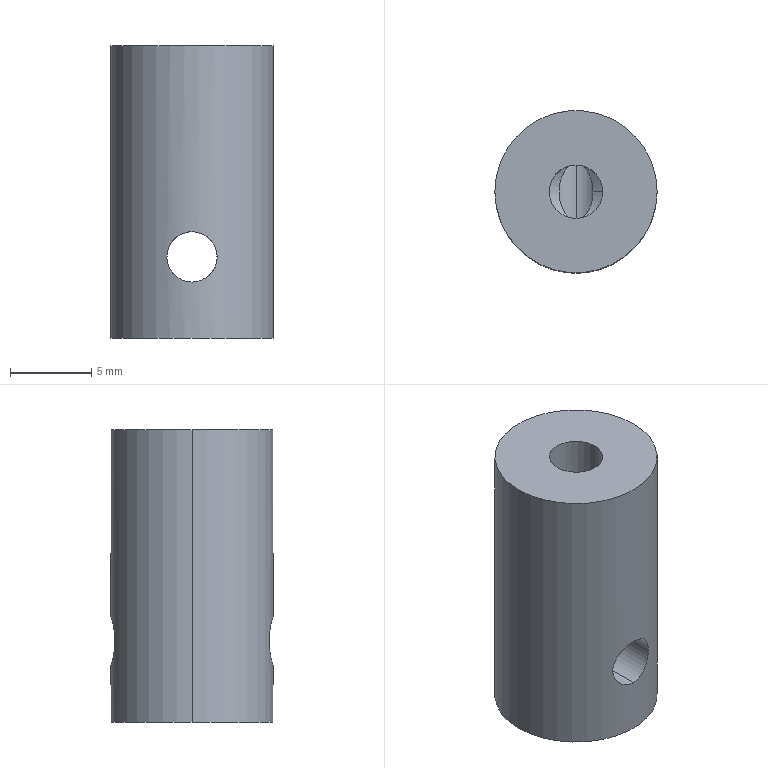Part | STEP file | push magnet union | 1 solid | 11 faces | box 10 x 10 x 18 mm | volume 1240 mm3 | cylinder 6 | cone 3 | plane 2 | commonest cylinder face diameters 3.1 x2 3.3 x2 10 x2